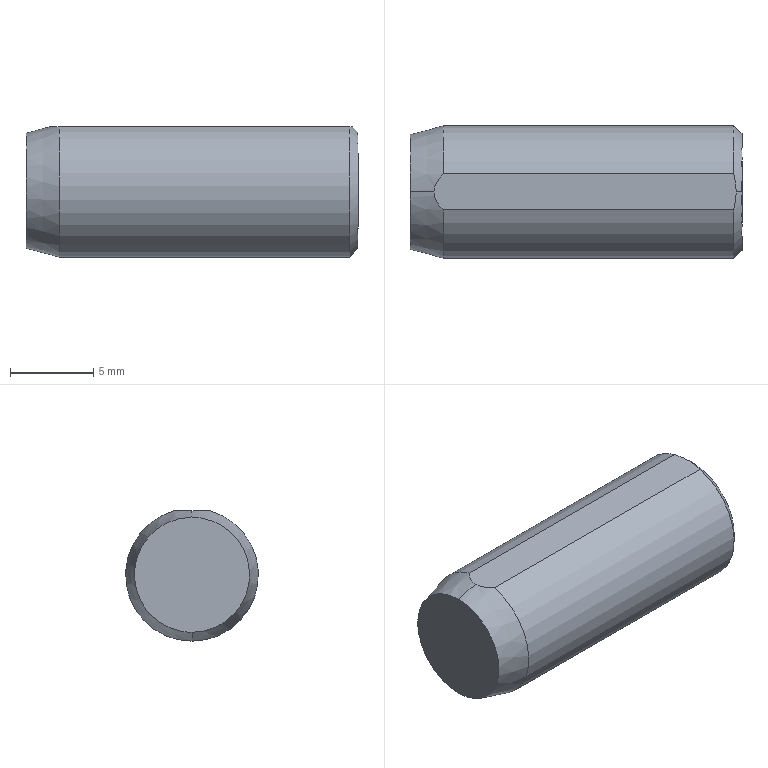Part | STEP file | MSTMS8-20 | 1 solid | 12 faces | box 20 x 8 x 7.85 mm | volume 827.27 mm3 | cone 6 | plane 3 | cylinder 3 | commonest cylinder face diameters 4.2 x2 8 x1
STEP:
#1=CARTESIAN_POINT('',(0.,0.,0.));
#2=DIRECTION('',(0.,0.,1.));
#3=DIRECTION('',(1.,0.,0.));
#4=AXIS2_PLACEMENT_3D('',#1,#2,#3);
#5=CARTESIAN_POINT('',(0.00003804,0.,-3.464));
#6=VERTEX_POINT('',#5);
#7=CARTESIAN_POINT('',(0.00003804,0.,3.464));
#8=VERTEX_POINT('',#7);
#9=CARTESIAN_POINT('',(0.00003804,0.,-3.464));
#10=CARTESIAN_POINT('',(0.,-0.9015,-3.475));
#11=CARTESIAN_POINT('',(0.,-1.808,-3.088));
#12=CARTESIAN_POINT('',(0.,-2.771,-2.129));
#13=CARTESIAN_POINT('',(0.,-3.026,-1.747));
#14=CARTESIAN_POINT('',(0.,-3.372,-0.9087));
#15=CARTESIAN_POINT('',(0.,-3.556,0.));
#16=CARTESIAN_POINT('',(0.,-3.372,0.9087));
#17=CARTESIAN_POINT('',(0.,-3.026,1.747));
#18=CARTESIAN_POINT('',(0.,-2.771,2.129));
#19=CARTESIAN_POINT('',(0.,-1.808,3.088));
#20=CARTESIAN_POINT('',(0.,-0.9015,3.475));
#21=CARTESIAN_POINT('',(0.00003804,0.,3.464));
#22=B_SPLINE_CURVE_WITH_KNOTS('',3,(#9,#10,#11,#12,#13,#14,#15,#16,#17,#18,#19,#20,#21),.UNSPECIFIED.,.F.,.F.,(4,2,2,1,2,2,4),(0.,0.25,0.375,0.5,0.625,0.75,1.),.UNSPECIFIED.);
#23=CARTESIAN_POINT('',(0.,-7.348,7.348));
#24=DIRECTION('',(1.,0.,0.));
#25=DIRECTION('',(0.,0.,-1.));
#26=AXIS2_PLACEMENT_3D('',#23,#24,#25);
#27=PLANE('',#26);
#28=CARTESIAN_POINT('',(10.812,7.348));
#29=CARTESIAN_POINT('',(10.823,6.447));
#30=CARTESIAN_POINT('',(10.436,5.54));
#31=CARTESIAN_POINT('',(9.477,4.577));
#32=CARTESIAN_POINT('',(9.095,4.322));
#33=CARTESIAN_POINT('',(8.257,3.976));
#34=CARTESIAN_POINT('',(7.348,3.792));
#35=CARTESIAN_POINT('',(6.439,3.976));
#36=CARTESIAN_POINT('',(5.601,4.322));
#37=CARTESIAN_POINT('',(5.219,4.577));
#38=CARTESIAN_POINT('',(4.26,5.54));
#39=CARTESIAN_POINT('',(3.873,6.447));
#40=CARTESIAN_POINT('',(3.884,7.348));
#41=B_SPLINE_CURVE_WITH_KNOTS('',3,(#28,#29,#30,#31,#32,#33,#34,#35,#36,#37,#38,#39,#40),.UNSPECIFIED.,.F.,.F.,(4,2,2,1,2,2,4),(0.,0.25,0.375,0.5,0.625,0.75,1.),.UNSPECIFIED.);
#42=(GEOMETRIC_REPRESENTATION_CONTEXT(2)PARAMETRIC_REPRESENTATION_CONTEXT()REPRESENTATION_CONTEXT('',''));
#43=DEFINITIONAL_REPRESENTATION('',(#41),#42);
#44=PCURVE('',#27,#43);
#45=CARTESIAN_POINT('',(-5.702,0.,0.));
#46=DIRECTION('',(1.,0.,0.));
#47=DIRECTION('',(0.,0.,-1.));
#48=AXIS2_PLACEMENT_3D('',#45,#46,#47);
#49=CONICAL_SURFACE('',#48,1.936,0.2618);
#50=CARTESIAN_POINT('',(6.283,5.702));
#51=CARTESIAN_POINT('',(6.26,5.702));
#52=CARTESIAN_POINT('',(6.212,5.702));
#53=CARTESIAN_POINT('',(6.141,5.702));
#54=CARTESIAN_POINT('',(6.07,5.702));
#55=CARTESIAN_POINT('',(5.999,5.702));
#56=CARTESIAN_POINT('',(5.927,5.702));
#57=CARTESIAN_POINT('',(5.856,5.701));
#58=CARTESIAN_POINT('',(5.784,5.701));
#59=CARTESIAN_POINT('',(5.712,5.701));
#60=CARTESIAN_POINT('',(5.64,5.701));
#61=CARTESIAN_POINT('',(5.569,5.702));
#62=CARTESIAN_POINT('',(5.498,5.702));
#63=CARTESIAN_POINT('',(5.426,5.702));
#64=CARTESIAN_POINT('',(5.355,5.702));
#65=CARTESIAN_POINT('',(5.284,5.702));
#66=CARTESIAN_POINT('',(5.213,5.702));
#67=CARTESIAN_POINT('',(5.142,5.702));
#68=CARTESIAN_POINT('',(5.07,5.702));
#69=CARTESIAN_POINT('',(4.999,5.702));
#70=CARTESIAN_POINT('',(4.927,5.702));
#71=CARTESIAN_POINT('',(4.856,5.702));
#72=CARTESIAN_POINT('',(4.784,5.702));
#73=CARTESIAN_POINT('',(4.712,5.702));
#74=CARTESIAN_POINT('',(4.641,5.702));
#75=CARTESIAN_POINT('',(4.569,5.702));
#76=CARTESIAN_POINT('',(4.498,5.702));
#77=CARTESIAN_POINT('',(4.426,5.702));
#78=CARTESIAN_POINT('',(4.355,5.702));
#79=CARTESIAN_POINT('',(4.283,5.702));
#80=CARTESIAN_POINT('',(4.212,5.702));
#81=CARTESIAN_POINT('',(4.141,5.702));
#82=CARTESIAN_POINT('',(4.07,5.702));
#83=CARTESIAN_POINT('',(3.998,5.702));
#84=CARTESIAN_POINT('',(3.927,5.702));
#85=CARTESIAN_POINT('',(3.856,5.702));
#86=CARTESIAN_POINT('',(3.784,5.701));
#87=CARTESIAN_POINT('',(3.713,5.701));
#88=CARTESIAN_POINT('',(3.641,5.701));
#89=CARTESIAN_POINT('',(3.569,5.701));
#90=CARTESIAN_POINT('',(3.498,5.702));
#91=CARTESIAN_POINT('',(3.426,5.702));
#92=CARTESIAN_POINT('',(3.355,5.702));
#93=CARTESIAN_POINT('',(3.284,5.702));
#94=CARTESIAN_POINT('',(3.213,5.702));
#95=CARTESIAN_POINT('',(3.165,5.702));
#96=CARTESIAN_POINT('',(3.142,5.702));
#97=B_SPLINE_CURVE_WITH_KNOTS('',3,(#50,#51,#52,#53,#54,#55,#56,#57,#58,#59,#60,#61,#62,#63,#64,#65,#66,#67,#68,#69,#70,#71,#72,#73,#74,#75,#76,#77,#78,#79,#80,#81,#82,#83,#84,#85,#86,#87,#88,#89,#90,#91,#92,#93,#94,#95,#96),.UNSPECIFIED.,.F.,.F.,(4,1,1,1,1,1,1,1,1,1,1,1,1,1,1,1,1,1,1,1,1,1,1,1,1,1,1,1,1,1,1,1,1,1,1,1,1,1,1,1,1,1,1,1,4),(0.,0.02273,0.04545,0.06818,0.09091,0.1136,0.1364,0.1591,0.1818,0.2045,0.2273,0.25,0.2727,0.2955,0.3182,0.3409,0.3636,0.3864,0.4091,0.4318,0.4545,0.4773,0.5,0.5227,0.5455,0.5682,0.5909,0.6136,0.6364,0.6591,0.6818,0.7045,0.7273,0.75,0.7727,0.7955,0.8182,0.8409,0.8636,0.8864,0.9091,0.9318,0.9545,0.9773,1.),.QUASI_UNIFORM_KNOTS.);
#98=(GEOMETRIC_REPRESENTATION_CONTEXT(2)PARAMETRIC_REPRESENTATION_CONTEXT()REPRESENTATION_CONTEXT('',''));
#99=DEFINITIONAL_REPRESENTATION('',(#97),#98);
#100=PCURVE('',#49,#99);
#101=SURFACE_CURVE('',#22,(#44,#100),.PCURVE_S1.);
#102=EDGE_CURVE('',#6,#8,#101,.T.);
#103=ORIENTED_EDGE('',*,*,#102,.F.);
#104=CARTESIAN_POINT('',(0.00003804,0.,3.464));
#105=CARTESIAN_POINT('',(0.,0.9015,3.475));
#106=CARTESIAN_POINT('',(0.,1.808,3.088));
#107=CARTESIAN_POINT('',(0.,2.771,2.129));
#108=CARTESIAN_POINT('',(0.,3.026,1.747));
#109=CARTESIAN_POINT('',(0.,3.372,0.9087));
#110=CARTESIAN_POINT('',(0.,3.556,0.));
#111=CARTESIAN_POINT('',(0.,3.372,-0.9087));
#112=CARTESIAN_POINT('',(0.,3.026,-1.747));
#113=CARTESIAN_POINT('',(0.,2.771,-2.129));
#114=CARTESIAN_POINT('',(0.,1.808,-3.088));
#115=CARTESIAN_POINT('',(0.,0.9015,-3.475));
#116=CARTESIAN_POINT('',(0.00003804,0.,-3.464));
#117=B_SPLINE_CURVE_WITH_KNOTS('',3,(#104,#105,#106,#107,#108,#109,#110,#111,#112,#113,#114,#115,#116),.UNSPECIFIED.,.F.,.F.,(4,2,2,1,2,2,4),(0.,0.25,0.375,0.5,0.625,0.75,1.),.UNSPECIFIED.);
#118=CARTESIAN_POINT('',(3.884,7.348));
#119=CARTESIAN_POINT('',(3.873,8.25));
#120=CARTESIAN_POINT('',(4.26,9.156));
#121=CARTESIAN_POINT('',(5.219,10.119));
#122=CARTESIAN_POINT('',(5.601,10.374));
#123=CARTESIAN_POINT('',(6.439,10.72));
#124=CARTESIAN_POINT('',(7.348,10.904));
#125=CARTESIAN_POINT('',(8.257,10.72));
#126=CARTESIAN_POINT('',(9.095,10.374));
#127=CARTESIAN_POINT('',(9.477,10.119));
#128=CARTESIAN_POINT('',(10.436,9.156));
#129=CARTESIAN_POINT('',(10.823,8.25));
#130=CARTESIAN_POINT('',(10.812,7.348));
#131=B_SPLINE_CURVE_WITH_KNOTS('',3,(#118,#119,#120,#121,#122,#123,#124,#125,#126,#127,#128,#129,#130),.UNSPECIFIED.,.F.,.F.,(4,2,2,1,2,2,4),(0.,0.25,0.375,0.5,0.625,0.75,1.),.UNSPECIFIED.);
#132=(GEOMETRIC_REPRESENTATION_CONTEXT(2)PARAMETRIC_REPRESENTATION_CONTEXT()REPRESENTATION_CONTEXT('',''));
#133=DEFINITIONAL_REPRESENTATION('',(#131),#132);
#134=PCURVE('',#27,#133);
#135=CARTESIAN_POINT('',(-5.702,0.,0.));
#136=DIRECTION('',(1.,0.,0.));
#137=DIRECTION('',(0.,0.,-1.));
#138=AXIS2_PLACEMENT_3D('',#135,#136,#137);
#139=CONICAL_SURFACE('',#138,1.936,0.2618);
#140=CARTESIAN_POINT('',(3.142,5.702));
#141=CARTESIAN_POINT('',(3.118,5.702));
#142=CARTESIAN_POINT('',(3.071,5.702));
#143=CARTESIAN_POINT('',(3.,5.702));
#144=CARTESIAN_POINT('',(2.928,5.702));
#145=CARTESIAN_POINT('',(2.857,5.702));
#146=CARTESIAN_POINT('',(2.786,5.702));
#147=CARTESIAN_POINT('',(2.714,5.701));
#148=CARTESIAN_POINT('',(2.642,5.701));
#149=CARTESIAN_POINT('',(2.571,5.701));
#150=CARTESIAN_POINT('',(2.499,5.701));
#151=CARTESIAN_POINT('',(2.427,5.702));
#152=CARTESIAN_POINT('',(2.356,5.702));
#153=CARTESIAN_POINT('',(2.285,5.702));
#154=CARTESIAN_POINT('',(2.214,5.702));
#155=CARTESIAN_POINT('',(2.142,5.702));
#156=CARTESIAN_POINT('',(2.071,5.702));
#157=CARTESIAN_POINT('',(2.,5.702));
#158=CARTESIAN_POINT('',(1.929,5.702));
#159=CARTESIAN_POINT('',(1.857,5.702));
#160=CARTESIAN_POINT('',(1.785,5.702));
#161=CARTESIAN_POINT('',(1.714,5.702));
#162=CARTESIAN_POINT('',(1.642,5.702));
#163=CARTESIAN_POINT('',(1.571,5.702));
#164=CARTESIAN_POINT('',(1.499,5.702));
#165=CARTESIAN_POINT('',(1.428,5.702));
#166=CARTESIAN_POINT('',(1.356,5.702));
#167=CARTESIAN_POINT('',(1.285,5.702));
#168=CARTESIAN_POINT('',(1.213,5.702));
#169=CARTESIAN_POINT('',(1.142,5.702));
#170=CARTESIAN_POINT('',(1.07,5.702));
#171=CARTESIAN_POINT('',(0.9992,5.702));
#172=CARTESIAN_POINT('',(0.9281,5.702));
#173=CARTESIAN_POINT('',(0.8569,5.702));
#174=CARTESIAN_POINT('',(0.7857,5.702));
#175=CARTESIAN_POINT('',(0.7143,5.702));
#176=CARTESIAN_POINT('',(0.6427,5.701));
#177=CARTESIAN_POINT('',(0.5711,5.701));
#178=CARTESIAN_POINT('',(0.4994,5.701));
#179=CARTESIAN_POINT('',(0.4276,5.701));
#180=CARTESIAN_POINT('',(0.356,5.702));
#181=CARTESIAN_POINT('',(0.2845,5.702));
#182=CARTESIAN_POINT('',(0.2132,5.702));
#183=CARTESIAN_POINT('',(0.142,5.702));
#184=CARTESIAN_POINT('',(0.07096,5.702));
#185=CARTESIAN_POINT('',(0.02365,5.702));
#186=CARTESIAN_POINT('',(0.,5.702));
#187=B_SPLINE_CURVE_WITH_KNOTS('',3,(#140,#141,#142,#143,#144,#145,#146,#147,#148,#149,#150,#151,#152,#153,#154,#155,#156,#157,#158,#159,#160,#161,#162,#163,#164,#165,#166,#167,#168,#169,#170,#171,#172,#173,#174,#175,#176,#177,#178,#179,#180,#181,#182,#183,#184,#185,#186),.UNSPECIFIED.,.F.,.F.,(4,1,1,1,1,1,1,1,1,1,1,1,1,1,1,1,1,1,1,1,1,1,1,1,1,1,1,1,1,1,1,1,1,1,1,1,1,1,1,1,1,1,1,1,4),(0.,0.02273,0.04545,0.06818,0.09091,0.1136,0.1364,0.1591,0.1818,0.2045,0.2273,0.25,0.2727,0.2955,0.3182,0.3409,0.3636,0.3864,0.4091,0.4318,0.4545,0.4773,0.5,0.5227,0.5455,0.5682,0.5909,0.6136,0.6364,0.6591,0.6818,0.7045,0.7273,0.75,0.7727,0.7955,0.8182,0.8409,0.8636,0.8864,0.9091,0.9318,0.9545,0.9773,1.),.QUASI_UNIFORM_KNOTS.);
#188=(GEOMETRIC_REPRESENTATION_CONTEXT(2)PARAMETRIC_REPRESENTATION_CONTEXT()REPRESENTATION_CONTEXT('',''));
#189=DEFINITIONAL_REPRESENTATION('',(#187),#188);
#190=PCURVE('',#139,#189);
#191=SURFACE_CURVE('',#117,(#134,#190),.PCURVE_S1.);
#192=EDGE_CURVE('',#8,#6,#191,.T.);
#193=ORIENTED_EDGE('',*,*,#192,.F.);
#194=EDGE_LOOP('',(#103,#193));
#195=FACE_BOUND('',#194,.F.);
#196=ADVANCED_FACE('',(#195),#27,.F.);
#197=CARTESIAN_POINT('',(1.441,0.00000021,3.85));
#198=VERTEX_POINT('',#197);
#199=CARTESIAN_POINT('',(0.00003804,0.,3.464));
#200=DIRECTION('',(0.9659,0.000000141,0.2588));
#201=VECTOR('',#200,1.);
#202=LINE('',#199,#201);
#203=CARTESIAN_POINT('',(3.142,5.702));
#204=DIRECTION('',(-0.000000038,1.));
#205=VECTOR('',#204,1.);
#206=LINE('',#203,#205);
#207=(GEOMETRIC_REPRESENTATION_CONTEXT(2)PARAMETRIC_REPRESENTATION_CONTEXT()REPRESENTATION_CONTEXT('',''));
#208=DEFINITIONAL_REPRESENTATION('',(#206),#207);
#209=PCURVE('',#49,#208);
#210=CARTESIAN_POINT('',(3.142,5.702));
#211=DIRECTION('',(-0.000000038,1.));
#212=VECTOR('',#211,1.);
#213=LINE('',#210,#212);
#214=(GEOMETRIC_REPRESENTATION_CONTEXT(2)PARAMETRIC_REPRESENTATION_CONTEXT()REPRESENTATION_CONTEXT('',''));
#215=DEFINITIONAL_REPRESENTATION('',(#213),#214);
#216=PCURVE('',#139,#215);
#217=SURFACE_CURVE('',#202,(#209,#216),.PCURVE_S1.);
#218=EDGE_CURVE('',#8,#198,#217,.T.);
#219=ORIENTED_EDGE('',*,*,#218,.F.);
#220=ORIENTED_EDGE('',*,*,#102,.F.);
#221=CARTESIAN_POINT('',(2.,-0.000000145,-4.));
#222=VERTEX_POINT('',#221);
#223=CARTESIAN_POINT('',(0.00003804,0.,-3.464));
#224=CARTESIAN_POINT('',(0.667,0.,-3.643));
#225=CARTESIAN_POINT('',(1.334,0.,-3.821));
#226=CARTESIAN_POINT('',(2.,-0.000000145,-4.));
#227=B_SPLINE_CURVE_WITH_KNOTS('',3,(#223,#224,#225,#226),.UNSPECIFIED.,.F.,.F.,(4,4),(0.,1.),.PIECEWISE_BEZIER_KNOTS.);
#228=CARTESIAN_POINT('',(6.283,5.702));
#229=CARTESIAN_POINT('',(6.283,5.732));
#230=CARTESIAN_POINT('',(6.283,5.793));
#231=CARTESIAN_POINT('',(6.283,5.884));
#232=CARTESIAN_POINT('',(6.283,5.975));
#233=CARTESIAN_POINT('',(6.283,6.066));
#234=CARTESIAN_POINT('',(6.283,6.157));
#235=CARTESIAN_POINT('',(6.283,6.247));
#236=CARTESIAN_POINT('',(6.283,6.338));
#237=CARTESIAN_POINT('',(6.283,6.429));
#238=CARTESIAN_POINT('',(6.283,6.52));
#239=CARTESIAN_POINT('',(6.283,6.611));
#240=CARTESIAN_POINT('',(6.283,6.702));
#241=CARTESIAN_POINT('',(6.283,6.793));
#242=CARTESIAN_POINT('',(6.283,6.884));
#243=CARTESIAN_POINT('',(6.283,6.975));
#244=CARTESIAN_POINT('',(6.283,7.066));
#245=CARTESIAN_POINT('',(6.283,7.157));
#246=CARTESIAN_POINT('',(6.283,7.248));
#247=CARTESIAN_POINT('',(6.283,7.338));
#248=CARTESIAN_POINT('',(6.283,7.429));
#249=CARTESIAN_POINT('',(6.283,7.52));
#250=CARTESIAN_POINT('',(6.283,7.611));
#251=CARTESIAN_POINT('',(6.283,7.672));
#252=CARTESIAN_POINT('',(6.283,7.702));
#253=B_SPLINE_CURVE_WITH_KNOTS('',3,(#228,#229,#230,#231,#232,#233,#234,#235,#236,#237,#238,#239,#240,#241,#242,#243,#244,#245,#246,#247,#248,#249,#250,#251,#252),.UNSPECIFIED.,.F.,.F.,(4,1,1,1,1,1,1,1,1,1,1,1,1,1,1,1,1,1,1,1,1,1,4),(0.,0.04545,0.09091,0.1364,0.1818,0.2273,0.2727,0.3182,0.3636,0.4091,0.4545,0.5,0.5455,0.5909,0.6364,0.6818,0.7273,0.7727,0.8182,0.8636,0.9091,0.9545,1.),.QUASI_UNIFORM_KNOTS.);
#254=(GEOMETRIC_REPRESENTATION_CONTEXT(2)PARAMETRIC_REPRESENTATION_CONTEXT()REPRESENTATION_CONTEXT('',''));
#255=DEFINITIONAL_REPRESENTATION('',(#253),#254);
#256=PCURVE('',#49,#255);
#257=CARTESIAN_POINT('',(0.,5.702));
#258=CARTESIAN_POINT('',(0.,5.732));
#259=CARTESIAN_POINT('',(0.,5.793));
#260=CARTESIAN_POINT('',(0.,5.884));
#261=CARTESIAN_POINT('',(0.,5.975));
#262=CARTESIAN_POINT('',(0.,6.066));
#263=CARTESIAN_POINT('',(0.,6.157));
#264=CARTESIAN_POINT('',(-0.000000001,6.247));
#265=CARTESIAN_POINT('',(-0.000000001,6.338));
#266=CARTESIAN_POINT('',(-0.000000002,6.429));
#267=CARTESIAN_POINT('',(-0.000000003,6.52));
#268=CARTESIAN_POINT('',(-0.000000004,6.611));
#269=CARTESIAN_POINT('',(-0.000000005,6.702));
#270=CARTESIAN_POINT('',(-0.000000006,6.793));
#271=CARTESIAN_POINT('',(-0.000000008,6.884));
#272=CARTESIAN_POINT('',(-0.00000001,6.975));
#273=CARTESIAN_POINT('',(-0.000000012,7.066));
#274=CARTESIAN_POINT('',(-0.000000014,7.157));
#275=CARTESIAN_POINT('',(-0.000000017,7.248));
#276=CARTESIAN_POINT('',(-0.00000002,7.338));
#277=CARTESIAN_POINT('',(-0.000000024,7.429));
#278=CARTESIAN_POINT('',(-0.000000028,7.52));
#279=CARTESIAN_POINT('',(-0.000000032,7.611));
#280=CARTESIAN_POINT('',(-0.000000035,7.672));
#281=CARTESIAN_POINT('',(-0.000000036,7.702));
#282=B_SPLINE_CURVE_WITH_KNOTS('',3,(#257,#258,#259,#260,#261,#262,#263,#264,#265,#266,#267,#268,#269,#270,#271,#272,#273,#274,#275,#276,#277,#278,#279,#280,#281),.UNSPECIFIED.,.F.,.F.,(4,1,1,1,1,1,1,1,1,1,1,1,1,1,1,1,1,1,1,1,1,1,4),(0.,0.04545,0.09091,0.1364,0.1818,0.2273,0.2727,0.3182,0.3636,0.4091,0.4545,0.5,0.5455,0.5909,0.6364,0.6818,0.7273,0.7727,0.8182,0.8636,0.9091,0.9545,1.),.QUASI_UNIFORM_KNOTS.);
#283=(GEOMETRIC_REPRESENTATION_CONTEXT(2)PARAMETRIC_REPRESENTATION_CONTEXT()REPRESENTATION_CONTEXT('',''));
#284=DEFINITIONAL_REPRESENTATION('',(#282),#283);
#285=PCURVE('',#139,#284);
#286=SURFACE_CURVE('',#227,(#256,#285),.PCURVE_S1.);
#287=EDGE_CURVE('',#6,#222,#286,.T.);
#288=ORIENTED_EDGE('',*,*,#287,.T.);
#289=CARTESIAN_POINT('',(2.001,-1.085,3.85));
#290=VERTEX_POINT('',#289);
#291=CARTESIAN_POINT('',(2.001,0.,0.));
#292=DIRECTION('',(-1.,0.,0.));
#293=DIRECTION('',(0.,-0.000000036,-1.));
#294=AXIS2_PLACEMENT_3D('',#291,#292,#293);
#295=CIRCLE('',#294,4.);
#296=CARTESIAN_POINT('',(6.283,7.703));
#297=DIRECTION('',(-1.,0.));
#298=VECTOR('',#297,1.);
#299=LINE('',#296,#298);
#300=(GEOMETRIC_REPRESENTATION_CONTEXT(2)PARAMETRIC_REPRESENTATION_CONTEXT()REPRESENTATION_CONTEXT('',''));
#301=DEFINITIONAL_REPRESENTATION('',(#299),#300);
#302=PCURVE('',#49,#301);
#303=CARTESIAN_POINT('',(10.75,0.,0.));
#304=DIRECTION('',(1.,0.,0.));
#305=DIRECTION('',(0.,0.008727,1.));
#306=AXIS2_PLACEMENT_3D('',#303,#304,#305);
#307=CYLINDRICAL_SURFACE('',#306,4.);
#308=CARTESIAN_POINT('',(3.15,-8.749));
#309=DIRECTION('',(-1.,0.));
#310=VECTOR('',#309,1.);
#311=LINE('',#308,#310);
#312=(GEOMETRIC_REPRESENTATION_CONTEXT(2)PARAMETRIC_REPRESENTATION_CONTEXT()REPRESENTATION_CONTEXT('',''));
#313=DEFINITIONAL_REPRESENTATION('',(#311),#312);
#314=PCURVE('',#307,#313);
#315=SURFACE_CURVE('',#295,(#302,#314),.PCURVE_S1.);
#316=EDGE_CURVE('',#222,#290,#315,.T.);
#317=ORIENTED_EDGE('',*,*,#316,.T.);
#318=CARTESIAN_POINT('',(1.441,0.00000021,3.85));
#319=CARTESIAN_POINT('',(1.441,-0.4288,3.85));
#320=CARTESIAN_POINT('',(1.711,-0.7982,3.85));
#321=CARTESIAN_POINT('',(2.001,-1.085,3.85));
#322=B_SPLINE_CURVE_WITH_KNOTS('',3,(#318,#319,#320,#321),.UNSPECIFIED.,.F.,.F.,(4,4),(0.,1.),.PIECEWISE_BEZIER_KNOTS.);
#323=CARTESIAN_POINT('',(3.142,7.143));
#324=CARTESIAN_POINT('',(3.147,7.143));
#325=CARTESIAN_POINT('',(3.157,7.144));
#326=CARTESIAN_POINT('',(3.172,7.149));
#327=CARTESIAN_POINT('',(3.186,7.157));
#328=CARTESIAN_POINT('',(3.201,7.167));
#329=CARTESIAN_POINT('',(3.215,7.181));
#330=CARTESIAN_POINT('',(3.229,7.197));
#331=CARTESIAN_POINT('',(3.243,7.216));
#332=CARTESIAN_POINT('',(3.256,7.237));
#333=CARTESIAN_POINT('',(3.269,7.261));
#334=CARTESIAN_POINT('',(3.282,7.286));
#335=CARTESIAN_POINT('',(3.295,7.314));
#336=CARTESIAN_POINT('',(3.308,7.343));
#337=CARTESIAN_POINT('',(3.32,7.374));
#338=CARTESIAN_POINT('',(3.332,7.406));
#339=CARTESIAN_POINT('',(3.343,7.44));
#340=CARTESIAN_POINT('',(3.355,7.475));
#341=CARTESIAN_POINT('',(3.366,7.511));
#342=CARTESIAN_POINT('',(3.376,7.548));
#343=CARTESIAN_POINT('',(3.387,7.586));
#344=CARTESIAN_POINT('',(3.397,7.624));
#345=CARTESIAN_POINT('',(3.407,7.663));
#346=CARTESIAN_POINT('',(3.413,7.689));
#347=CARTESIAN_POINT('',(3.416,7.703));
#348=B_SPLINE_CURVE_WITH_KNOTS('',3,(#323,#324,#325,#326,#327,#328,#329,#330,#331,#332,#333,#334,#335,#336,#337,#338,#339,#340,#341,#342,#343,#344,#345,#346,#347),.UNSPECIFIED.,.F.,.F.,(4,1,1,1,1,1,1,1,1,1,1,1,1,1,1,1,1,1,1,1,1,1,4),(0.,0.04545,0.09091,0.1364,0.1818,0.2273,0.2727,0.3182,0.3636,0.4091,0.4545,0.5,0.5455,0.5909,0.6364,0.6818,0.7273,0.7727,0.8182,0.8636,0.9091,0.9545,1.),.QUASI_UNIFORM_KNOTS.);
#349=(GEOMETRIC_REPRESENTATION_CONTEXT(2)PARAMETRIC_REPRESENTATION_CONTEXT()REPRESENTATION_CONTEXT('',''));
#350=DEFINITIONAL_REPRESENTATION('',(#348),#349);
#351=PCURVE('',#49,#350);
#352=CARTESIAN_POINT('',(-3.208,-13.753,3.85));
#353=DIRECTION('',(0.,0.,-1.));
#354=DIRECTION('',(0.,1.,0.));
#355=AXIS2_PLACEMENT_3D('',#352,#353,#354);
#356=PLANE('',#355);
#357=CARTESIAN_POINT('',(13.753,4.649));
#358=CARTESIAN_POINT('',(13.324,4.648));
#359=CARTESIAN_POINT('',(12.955,4.919));
#360=CARTESIAN_POINT('',(12.668,5.209));
#361=B_SPLINE_CURVE_WITH_KNOTS('',3,(#357,#358,#359,#360),.UNSPECIFIED.,.F.,.F.,(4,4),(0.,1.),.PIECEWISE_BEZIER_KNOTS.);
#362=(GEOMETRIC_REPRESENTATION_CONTEXT(2)PARAMETRIC_REPRESENTATION_CONTEXT()REPRESENTATION_CONTEXT('',''));
#363=DEFINITIONAL_REPRESENTATION('',(#361),#362);
#364=PCURVE('',#356,#363);
#365=SURFACE_CURVE('',#322,(#351,#364),.PCURVE_S1.);
#366=EDGE_CURVE('',#198,#290,#365,.T.);
#367=ORIENTED_EDGE('',*,*,#366,.F.);
#368=EDGE_LOOP('',(#219,#220,#288,#317,#367));
#369=FACE_BOUND('',#368,.T.);
#370=ADVANCED_FACE('',(#369),#49,.T.);
#371=CARTESIAN_POINT('',(19.65,0.000000117,3.85));
#372=VERTEX_POINT('',#371);
#373=CARTESIAN_POINT('',(19.5,1.085,3.85));
#374=VERTEX_POINT('',#373);
#375=CARTESIAN_POINT('',(19.65,0.000000117,3.85));
#376=CARTESIAN_POINT('',(19.65,0.3664,3.85));
#377=CARTESIAN_POINT('',(19.596,0.7319,3.85));
#378=CARTESIAN_POINT('',(19.5,1.085,3.85));
#379=B_SPLINE_CURVE_WITH_KNOTS('',3,(#375,#376,#377,#378),.UNSPECIFIED.,.F.,.F.,(4,4),(0.,1.),.PIECEWISE_BEZIER_KNOTS.);
#380=CARTESIAN_POINT('',(13.753,22.858));
#381=CARTESIAN_POINT('',(14.12,22.858));
#382=CARTESIAN_POINT('',(14.485,22.804));
#383=CARTESIAN_POINT('',(14.838,22.708));
#384=B_SPLINE_CURVE_WITH_KNOTS('',3,(#380,#381,#382,#383),.UNSPECIFIED.,.F.,.F.,(4,4),(0.,1.),.PIECEWISE_BEZIER_KNOTS.);
#385=(GEOMETRIC_REPRESENTATION_CONTEXT(2)PARAMETRIC_REPRESENTATION_CONTEXT()REPRESENTATION_CONTEXT('',''));
#386=DEFINITIONAL_REPRESENTATION('',(#384),#385);
#387=PCURVE('',#356,#386);
#388=CARTESIAN_POINT('',(-976.5,0.,0.));
#389=DIRECTION('',(-1.,0.,0.));
#390=DIRECTION('',(0.,0.,-1.));
#391=AXIS2_PLACEMENT_3D('',#388,#389,#390);
#392=CONICAL_SURFACE('',#391,999.941,0.7854);
#393=CARTESIAN_POINT('',(3.142,-996.15));
#394=CARTESIAN_POINT('',(3.146,-996.15));
#395=CARTESIAN_POINT('',(3.155,-996.15));
#396=CARTESIAN_POINT('',(3.168,-996.149));
#397=CARTESIAN_POINT('',(3.18,-996.147));
#398=CARTESIAN_POINT('',(3.193,-996.145));
#399=CARTESIAN_POINT('',(3.206,-996.142));
#400=CARTESIAN_POINT('',(3.219,-996.138));
#401=CARTESIAN_POINT('',(3.232,-996.134));
#402=CARTESIAN_POINT('',(3.245,-996.129));
#403=CARTESIAN_POINT('',(3.258,-996.124));
#404=CARTESIAN_POINT('',(3.27,-996.118));
#405=CARTESIAN_POINT('',(3.283,-996.111));
#406=CARTESIAN_POINT('',(3.295,-996.104));
#407=CARTESIAN_POINT('',(3.308,-996.096));
#408=CARTESIAN_POINT('',(3.32,-996.088));
#409=CARTESIAN_POINT('',(3.333,-996.079));
#410=CARTESIAN_POINT('',(3.345,-996.069));
#411=CARTESIAN_POINT('',(3.357,-996.059));
#412=CARTESIAN_POINT('',(3.369,-996.048));
#413=CARTESIAN_POINT('',(3.381,-996.037));
#414=CARTESIAN_POINT('',(3.393,-996.025));
#415=CARTESIAN_POINT('',(3.405,-996.013));
#416=CARTESIAN_POINT('',(3.412,-996.004));
#417=CARTESIAN_POINT('',(3.416,-996.));
#418=B_SPLINE_CURVE_WITH_KNOTS('',3,(#393,#394,#395,#396,#397,#398,#399,#400,#401,#402,#403,#404,#405,#406,#407,#408,#409,#410,#411,#412,#413,#414,#415,#416,#417),.UNSPECIFIED.,.F.,.F.,(4,1,1,1,1,1,1,1,1,1,1,1,1,1,1,1,1,1,1,1,1,1,4),(0.,0.04545,0.09091,0.1364,0.1818,0.2273,0.2727,0.3182,0.3636,0.4091,0.4545,0.5,0.5455,0.5909,0.6364,0.6818,0.7273,0.7727,0.8182,0.8636,0.9091,0.9545,1.),.QUASI_UNIFORM_KNOTS.);
#419=(GEOMETRIC_REPRESENTATION_CONTEXT(2)PARAMETRIC_REPRESENTATION_CONTEXT()REPRESENTATION_CONTEXT('',''));
#420=DEFINITIONAL_REPRESENTATION('',(#418),#419);
#421=PCURVE('',#392,#420);
#422=SURFACE_CURVE('',#379,(#387,#421),.PCURVE_S1.);
#423=EDGE_CURVE('',#372,#374,#422,.T.);
#424=ORIENTED_EDGE('',*,*,#423,.F.);
#425=CARTESIAN_POINT('',(19.5,-1.085,3.85));
#426=VERTEX_POINT('',#425);
#427=CARTESIAN_POINT('',(19.5,-1.085,3.85));
#428=CARTESIAN_POINT('',(19.596,-0.7319,3.85));
#429=CARTESIAN_POINT('',(19.65,-0.3664,3.85));
#430=CARTESIAN_POINT('',(19.65,0.000000117,3.85));
#431=B_SPLINE_CURVE_WITH_KNOTS('',3,(#427,#428,#429,#430),.UNSPECIFIED.,.F.,.F.,(4,4),(0.,1.),.PIECEWISE_BEZIER_KNOTS.);
#432=CARTESIAN_POINT('',(12.668,22.708));
#433=CARTESIAN_POINT('',(13.021,22.804));
#434=CARTESIAN_POINT('',(13.387,22.858));
#435=CARTESIAN_POINT('',(13.753,22.858));
#436=B_SPLINE_CURVE_WITH_KNOTS('',3,(#432,#433,#434,#435),.UNSPECIFIED.,.F.,.F.,(4,4),(0.,1.),.PIECEWISE_BEZIER_KNOTS.);
#437=(GEOMETRIC_REPRESENTATION_CONTEXT(2)PARAMETRIC_REPRESENTATION_CONTEXT()REPRESENTATION_CONTEXT('',''));
#438=DEFINITIONAL_REPRESENTATION('',(#436),#437);
#439=PCURVE('',#356,#438);
#440=CARTESIAN_POINT('',(-976.5,0.,0.));
#441=DIRECTION('',(-1.,0.,0.));
#442=DIRECTION('',(0.,0.,-1.));
#443=AXIS2_PLACEMENT_3D('',#440,#441,#442);
#444=CONICAL_SURFACE('',#443,999.941,0.7854);
#445=CARTESIAN_POINT('',(2.867,-996.));
#446=CARTESIAN_POINT('',(2.871,-996.004));
#447=CARTESIAN_POINT('',(2.878,-996.013));
#448=CARTESIAN_POINT('',(2.89,-996.025));
#449=CARTESIAN_POINT('',(2.902,-996.037));
#450=CARTESIAN_POINT('',(2.914,-996.048));
#451=CARTESIAN_POINT('',(2.926,-996.059));
#452=CARTESIAN_POINT('',(2.938,-996.069));
#453=CARTESIAN_POINT('',(2.951,-996.079));
#454=CARTESIAN_POINT('',(2.963,-996.088));
#455=CARTESIAN_POINT('',(2.975,-996.096));
#456=CARTESIAN_POINT('',(2.988,-996.104));
#457=CARTESIAN_POINT('',(3.,-996.111));
#458=CARTESIAN_POINT('',(3.013,-996.118));
#459=CARTESIAN_POINT('',(3.026,-996.124));
#460=CARTESIAN_POINT('',(3.038,-996.129));
#461=CARTESIAN_POINT('',(3.051,-996.134));
#462=CARTESIAN_POINT('',(3.064,-996.138));
#463=CARTESIAN_POINT('',(3.077,-996.142));
#464=CARTESIAN_POINT('',(3.09,-996.145));
#465=CARTESIAN_POINT('',(3.103,-996.147));
#466=CARTESIAN_POINT('',(3.116,-996.149));
#467=CARTESIAN_POINT('',(3.129,-996.15));
#468=CARTESIAN_POINT('',(3.137,-996.15));
#469=CARTESIAN_POINT('',(3.142,-996.15));
#470=B_SPLINE_CURVE_WITH_KNOTS('',3,(#445,#446,#447,#448,#449,#450,#451,#452,#453,#454,#455,#456,#457,#458,#459,#460,#461,#462,#463,#464,#465,#466,#467,#468,#469),.UNSPECIFIED.,.F.,.F.,(4,1,1,1,1,1,1,1,1,1,1,1,1,1,1,1,1,1,1,1,1,1,4),(0.,0.04545,0.09091,0.1364,0.1818,0.2273,0.2727,0.3182,0.3636,0.4091,0.4545,0.5,0.5455,0.5909,0.6364,0.6818,0.7273,0.7727,0.8182,0.8636,0.9091,0.9545,1.),.QUASI_UNIFORM_KNOTS.);
#471=(GEOMETRIC_REPRESENTATION_CONTEXT(2)PARAMETRIC_REPRESENTATION_CONTEXT()REPRESENTATION_CONTEXT('',''));
#472=DEFINITIONAL_REPRESENTATION('',(#470),#471);
#473=PCURVE('',#444,#472);
#474=SURFACE_CURVE('',#431,(#439,#473),.PCURVE_S1.);
#475=EDGE_CURVE('',#426,#372,#474,.T.);
#476=ORIENTED_EDGE('',*,*,#475,.F.);
#477=CARTESIAN_POINT('',(2.001,-1.085,3.85));
#478=DIRECTION('',(1.,0.,0.));
#479=VECTOR('',#478,1.);
#480=LINE('',#477,#479);
#481=CARTESIAN_POINT('',(12.668,5.209));
#482=DIRECTION('',(0.,1.));
#483=VECTOR('',#482,1.);
#484=LINE('',#481,#483);
#485=(GEOMETRIC_REPRESENTATION_CONTEXT(2)PARAMETRIC_REPRESENTATION_CONTEXT()REPRESENTATION_CONTEXT('',''));
#486=DEFINITIONAL_REPRESENTATION('',(#484),#485);
#487=PCURVE('',#356,#486);
#488=CARTESIAN_POINT('',(0.2835,-8.749));
#489=DIRECTION('',(0.,1.));
#490=VECTOR('',#489,1.);
#491=LINE('',#488,#490);
#492=(GEOMETRIC_REPRESENTATION_CONTEXT(2)PARAMETRIC_REPRESENTATION_CONTEXT()REPRESENTATION_CONTEXT('',''));
#493=DEFINITIONAL_REPRESENTATION('',(#491),#492);
#494=PCURVE('',#307,#493);
#495=SURFACE_CURVE('',#480,(#487,#494),.PCURVE_S1.);
#496=EDGE_CURVE('',#290,#426,#495,.T.);
#497=ORIENTED_EDGE('',*,*,#496,.F.);
#498=ORIENTED_EDGE('',*,*,#366,.F.);
#499=CARTESIAN_POINT('',(2.001,1.085,3.85));
#500=VERTEX_POINT('',#499);
#501=CARTESIAN_POINT('',(2.001,1.085,3.85));
#502=CARTESIAN_POINT('',(1.711,0.7982,3.85));
#503=CARTESIAN_POINT('',(1.441,0.4288,3.85));
#504=CARTESIAN_POINT('',(1.441,0.00000021,3.85));
#505=B_SPLINE_CURVE_WITH_KNOTS('',3,(#501,#502,#503,#504),.UNSPECIFIED.,.F.,.F.,(4,4),(0.,1.),.PIECEWISE_BEZIER_KNOTS.);
#506=CARTESIAN_POINT('',(14.838,5.209));
#507=CARTESIAN_POINT('',(14.551,4.919));
#508=CARTESIAN_POINT('',(14.182,4.648));
#509=CARTESIAN_POINT('',(13.753,4.649));
#510=B_SPLINE_CURVE_WITH_KNOTS('',3,(#506,#507,#508,#509),.UNSPECIFIED.,.F.,.F.,(4,4),(0.,1.),.PIECEWISE_BEZIER_KNOTS.);
#511=(GEOMETRIC_REPRESENTATION_CONTEXT(2)PARAMETRIC_REPRESENTATION_CONTEXT()REPRESENTATION_CONTEXT('',''));
#512=DEFINITIONAL_REPRESENTATION('',(#510),#511);
#513=PCURVE('',#356,#512);
#514=CARTESIAN_POINT('',(2.867,7.703));
#515=CARTESIAN_POINT('',(2.87,7.689));
#516=CARTESIAN_POINT('',(2.876,7.663));
#517=CARTESIAN_POINT('',(2.886,7.624));
#518=CARTESIAN_POINT('',(2.896,7.586));
#519=CARTESIAN_POINT('',(2.907,7.548));
#520=CARTESIAN_POINT('',(2.918,7.511));
#521=CARTESIAN_POINT('',(2.929,7.475));
#522=CARTESIAN_POINT('',(2.94,7.44));
#523=CARTESIAN_POINT('',(2.952,7.406));
#524=CARTESIAN_POINT('',(2.963,7.374));
#525=CARTESIAN_POINT('',(2.976,7.343));
#526=CARTESIAN_POINT('',(2.988,7.314));
#527=CARTESIAN_POINT('',(3.001,7.286));
#528=CARTESIAN_POINT('',(3.014,7.261));
#529=CARTESIAN_POINT('',(3.027,7.237));
#530=CARTESIAN_POINT('',(3.04,7.216));
#531=CARTESIAN_POINT('',(3.054,7.197));
#532=CARTESIAN_POINT('',(3.068,7.181));
#533=CARTESIAN_POINT('',(3.082,7.167));
#534=CARTESIAN_POINT('',(3.097,7.157));
#535=CARTESIAN_POINT('',(3.112,7.149));
#536=CARTESIAN_POINT('',(3.126,7.144));
#537=CARTESIAN_POINT('',(3.137,7.143));
#538=CARTESIAN_POINT('',(3.142,7.143));
#539=B_SPLINE_CURVE_WITH_KNOTS('',3,(#514,#515,#516,#517,#518,#519,#520,#521,#522,#523,#524,#525,#526,#527,#528,#529,#530,#531,#532,#533,#534,#535,#536,#537,#538),.UNSPECIFIED.,.F.,.F.,(4,1,1,1,1,1,1,1,1,1,1,1,1,1,1,1,1,1,1,1,1,1,4),(0.,0.04545,0.09091,0.1364,0.1818,0.2273,0.2727,0.3182,0.3636,0.4091,0.4545,0.5,0.5455,0.5909,0.6364,0.6818,0.7273,0.7727,0.8182,0.8636,0.9091,0.9545,1.),.QUASI_UNIFORM_KNOTS.);
#540=(GEOMETRIC_REPRESENTATION_CONTEXT(2)PARAMETRIC_REPRESENTATION_CONTEXT()REPRESENTATION_CONTEXT('',''));
#541=DEFINITIONAL_REPRESENTATION('',(#539),#540);
#542=PCURVE('',#139,#541);
#543=SURFACE_CURVE('',#505,(#513,#542),.PCURVE_S1.);
#544=EDGE_CURVE('',#500,#198,#543,.T.);
#545=ORIENTED_EDGE('',*,*,#544,.F.);
#546=CARTESIAN_POINT('',(2.001,1.085,3.85));
#547=DIRECTION('',(1.,0.,0.));
#548=VECTOR('',#547,1.);
#549=LINE('',#546,#548);
#550=CARTESIAN_POINT('',(14.838,5.209));
#551=DIRECTION('',(0.,1.));
#552=VECTOR('',#551,1.);
#553=LINE('',#550,#552);
#554=(GEOMETRIC_REPRESENTATION_CONTEXT(2)PARAMETRIC_REPRESENTATION_CONTEXT()REPRESENTATION_CONTEXT('',''));
#555=DEFINITIONAL_REPRESENTATION('',(#553),#554);
#556=PCURVE('',#356,#555);
#557=CARTESIAN_POINT('',(6.017,-8.749));
#558=DIRECTION('',(0.,1.));
#559=VECTOR('',#558,1.);
#560=LINE('',#557,#559);
#561=(GEOMETRIC_REPRESENTATION_CONTEXT(2)PARAMETRIC_REPRESENTATION_CONTEXT()REPRESENTATION_CONTEXT('',''));
#562=DEFINITIONAL_REPRESENTATION('',(#560),#561);
#563=PCURVE('',#307,#562);
#564=SURFACE_CURVE('',#549,(#556,#563),.PCURVE_S1.);
#565=EDGE_CURVE('',#500,#374,#564,.T.);
#566=ORIENTED_EDGE('',*,*,#565,.T.);
#567=EDGE_LOOP('',(#424,#476,#497,#498,#545,#566));
#568=FACE_BOUND('',#567,.F.);
#569=ADVANCED_FACE('',(#568),#356,.F.);
#570=CARTESIAN_POINT('',(20.,0.,3.5));
#571=VERTEX_POINT('',#570);
#572=CARTESIAN_POINT('',(20.,0.,3.5));
#573=DIRECTION('',(-0.7071,0.000000236,0.7071));
#574=VECTOR('',#573,1.);
#575=LINE('',#572,#574);
#576=CARTESIAN_POINT('',(3.142,-996.5));
#577=DIRECTION('',(0.000000087,1.));
#578=VECTOR('',#577,1.);
#579=LINE('',#576,#578);
#580=(GEOMETRIC_REPRESENTATION_CONTEXT(2)PARAMETRIC_REPRESENTATION_CONTEXT()REPRESENTATION_CONTEXT('',''));
#581=DEFINITIONAL_REPRESENTATION('',(#579),#580);
#582=PCURVE('',#392,#581);
#583=CARTESIAN_POINT('',(3.142,-996.5));
#584=DIRECTION('',(0.000000087,1.));
#585=VECTOR('',#584,1.);
#586=LINE('',#583,#585);
#587=(GEOMETRIC_REPRESENTATION_CONTEXT(2)PARAMETRIC_REPRESENTATION_CONTEXT()REPRESENTATION_CONTEXT('',''));
#588=DEFINITIONAL_REPRESENTATION('',(#586),#587);
#589=PCURVE('',#444,#588);
#590=SURFACE_CURVE('',#575,(#582,#589),.PCURVE_S1.);
#591=EDGE_CURVE('',#571,#372,#590,.T.);
#592=ORIENTED_EDGE('',*,*,#591,.F.);
#593=CARTESIAN_POINT('',(20.,0.,-3.5));
#594=VERTEX_POINT('',#593);
#595=CARTESIAN_POINT('',(20.,0.,-3.5));
#596=CARTESIAN_POINT('',(20.,0.9108,-3.511));
#597=CARTESIAN_POINT('',(20.,1.827,-3.12));
#598=CARTESIAN_POINT('',(20.,2.8,-2.151));
#599=CARTESIAN_POINT('',(20.,3.057,-1.765));
#600=CARTESIAN_POINT('',(20.,3.407,-0.9182));
#601=CARTESIAN_POINT('',(20.,3.593,0.));
#602=CARTESIAN_POINT('',(20.,3.407,0.9182));
#603=CARTESIAN_POINT('',(20.,3.057,1.765));
#604=CARTESIAN_POINT('',(20.,2.8,2.151));
#605=CARTESIAN_POINT('',(20.,1.827,3.12));
#606=CARTESIAN_POINT('',(20.,0.9108,3.511));
#607=CARTESIAN_POINT('',(20.,0.,3.5));
#608=B_SPLINE_CURVE_WITH_KNOTS('',3,(#595,#596,#597,#598,#599,#600,#601,#602,#603,#604,#605,#606,#607),.UNSPECIFIED.,.F.,.F.,(4,2,2,1,2,2,4),(0.,0.25,0.375,0.5,0.625,0.75,1.),.UNSPECIFIED.);
#609=CARTESIAN_POINT('',(6.283,-996.5));
#610=CARTESIAN_POINT('',(6.26,-996.499));
#611=CARTESIAN_POINT('',(6.212,-996.499));
#612=CARTESIAN_POINT('',(6.141,-996.499));
#613=CARTESIAN_POINT('',(6.07,-996.499));
#614=CARTESIAN_POINT('',(5.999,-996.5));
#615=CARTESIAN_POINT('',(5.927,-996.5));
#616=CARTESIAN_POINT('',(5.856,-996.501));
#617=CARTESIAN_POINT('',(5.784,-996.501));
#618=CARTESIAN_POINT('',(5.712,-996.501));
#619=CARTESIAN_POINT('',(5.64,-996.501));
#620=CARTESIAN_POINT('',(5.569,-996.5));
#621=CARTESIAN_POINT('',(5.498,-996.5));
#622=CARTESIAN_POINT('',(5.426,-996.5));
#623=CARTESIAN_POINT('',(5.355,-996.5));
#624=CARTESIAN_POINT('',(5.284,-996.5));
#625=CARTESIAN_POINT('',(5.213,-996.5));
#626=CARTESIAN_POINT('',(5.142,-996.5));
#627=CARTESIAN_POINT('',(5.07,-996.5));
#628=CARTESIAN_POINT('',(4.999,-996.5));
#629=CARTESIAN_POINT('',(4.927,-996.5));
#630=CARTESIAN_POINT('',(4.856,-996.5));
#631=CARTESIAN_POINT('',(4.784,-996.5));
#632=CARTESIAN_POINT('',(4.712,-996.5));
#633=CARTESIAN_POINT('',(4.641,-996.5));
#634=CARTESIAN_POINT('',(4.569,-996.5));
#635=CARTESIAN_POINT('',(4.498,-996.5));
#636=CARTESIAN_POINT('',(4.426,-996.5));
#637=CARTESIAN_POINT('',(4.355,-996.5));
#638=CARTESIAN_POINT('',(4.283,-996.5));
#639=CARTESIAN_POINT('',(4.212,-996.5));
#640=CARTESIAN_POINT('',(4.141,-996.5));
#641=CARTESIAN_POINT('',(4.07,-996.5));
#642=CARTESIAN_POINT('',(3.998,-996.5));
#643=CARTESIAN_POINT('',(3.927,-996.5));
#644=CARTESIAN_POINT('',(3.856,-996.5));
#645=CARTESIAN_POINT('',(3.784,-996.501));
#646=CARTESIAN_POINT('',(3.713,-996.501));
#647=CARTESIAN_POINT('',(3.641,-996.501));
#648=CARTESIAN_POINT('',(3.569,-996.501));
#649=CARTESIAN_POINT('',(3.498,-996.5));
#650=CARTESIAN_POINT('',(3.426,-996.5));
#651=CARTESIAN_POINT('',(3.355,-996.499));
#652=CARTESIAN_POINT('',(3.284,-996.499));
#653=CARTESIAN_POINT('',(3.213,-996.499));
#654=CARTESIAN_POINT('',(3.165,-996.499));
#655=CARTESIAN_POINT('',(3.142,-996.5));
#656=B_SPLINE_CURVE_WITH_KNOTS('',3,(#609,#610,#611,#612,#613,#614,#615,#616,#617,#618,#619,#620,#621,#622,#623,#624,#625,#626,#627,#628,#629,#630,#631,#632,#633,#634,#635,#636,#637,#638,#639,#640,#641,#642,#643,#644,#645,#646,#647,#648,#649,#650,#651,#652,#653,#654,#655),.UNSPECIFIED.,.F.,.F.,(4,1,1,1,1,1,1,1,1,1,1,1,1,1,1,1,1,1,1,1,1,1,1,1,1,1,1,1,1,1,1,1,1,1,1,1,1,1,1,1,1,1,1,1,4),(0.,0.02273,0.04545,0.06818,0.09091,0.1136,0.1364,0.1591,0.1818,0.2045,0.2273,0.25,0.2727,0.2955,0.3182,0.3409,0.3636,0.3864,0.4091,0.4318,0.4545,0.4773,0.5,0.5227,0.5455,0.5682,0.5909,0.6136,0.6364,0.6591,0.6818,0.7045,0.7273,0.75,0.7727,0.7955,0.8182,0.8409,0.8636,0.8864,0.9091,0.9318,0.9545,0.9773,1.),.QUASI_UNIFORM_KNOTS.);
#657=(GEOMETRIC_REPRESENTATION_CONTEXT(2)PARAMETRIC_REPRESENTATION_CONTEXT()REPRESENTATION_CONTEXT('',''));
#658=DEFINITIONAL_REPRESENTATION('',(#656),#657);
#659=PCURVE('',#392,#658);
#660=CARTESIAN_POINT('',(20.,-7.424,7.424));
#661=DIRECTION('',(1.,0.,0.));
#662=DIRECTION('',(0.,0.,-1.));
#663=AXIS2_PLACEMENT_3D('',#660,#661,#662);
#664=PLANE('',#663);
#665=CARTESIAN_POINT('',(10.924,7.424));
#666=CARTESIAN_POINT('',(10.935,8.335));
#667=CARTESIAN_POINT('',(10.544,9.251));
#668=CARTESIAN_POINT('',(9.576,10.224));
#669=CARTESIAN_POINT('',(9.189,10.482));
#670=CARTESIAN_POINT('',(8.343,10.831));
#671=CARTESIAN_POINT('',(7.424,11.017));
#672=CARTESIAN_POINT('',(6.506,10.831));
#673=CARTESIAN_POINT('',(5.659,10.482));
#674=CARTESIAN_POINT('',(5.273,10.224));
#675=CARTESIAN_POINT('',(4.305,9.251));
#676=CARTESIAN_POINT('',(3.914,8.335));
#677=CARTESIAN_POINT('',(3.924,7.424));
#678=B_SPLINE_CURVE_WITH_KNOTS('',3,(#665,#666,#667,#668,#669,#670,#671,#672,#673,#674,#675,#676,#677),.UNSPECIFIED.,.F.,.F.,(4,2,2,1,2,2,4),(0.,0.25,0.375,0.5,0.625,0.75,1.),.UNSPECIFIED.);
#679=(GEOMETRIC_REPRESENTATION_CONTEXT(2)PARAMETRIC_REPRESENTATION_CONTEXT()REPRESENTATION_CONTEXT('',''));
#680=DEFINITIONAL_REPRESENTATION('',(#678),#679);
#681=PCURVE('',#664,#680);
#682=SURFACE_CURVE('',#608,(#659,#681),.PCURVE_S1.);
#683=EDGE_CURVE('',#594,#571,#682,.T.);
#684=ORIENTED_EDGE('',*,*,#683,.F.);
#685=CARTESIAN_POINT('',(19.5,-0.000000081,-4.));
#686=VERTEX_POINT('',#685);
#687=CARTESIAN_POINT('',(20.,0.,-3.5));
#688=CARTESIAN_POINT('',(19.833,0.,-3.667));
#689=CARTESIAN_POINT('',(19.666,0.,-3.833));
#690=CARTESIAN_POINT('',(19.5,-0.000000081,-4.));
#691=B_SPLINE_CURVE_WITH_KNOTS('',3,(#687,#688,#689,#690),.UNSPECIFIED.,.F.,.F.,(4,4),(0.,1.),.PIECEWISE_BEZIER_KNOTS.);
#692=CARTESIAN_POINT('',(6.283,-996.5));
#693=CARTESIAN_POINT('',(6.283,-996.492));
#694=CARTESIAN_POINT('',(6.283,-996.477));
#695=CARTESIAN_POINT('',(6.283,-996.454));
#696=CARTESIAN_POINT('',(6.283,-996.432));
#697=CARTESIAN_POINT('',(6.283,-996.409));
#698=CARTESIAN_POINT('',(6.283,-996.386));
#699=CARTESIAN_POINT('',(6.283,-996.364));
#700=CARTESIAN_POINT('',(6.283,-996.341));
#701=CARTESIAN_POINT('',(6.283,-996.318));
#702=CARTESIAN_POINT('',(6.283,-996.295));
#703=CARTESIAN_POINT('',(6.283,-996.273));
#704=CARTESIAN_POINT('',(6.283,-996.25));
#705=CARTESIAN_POINT('',(6.283,-996.227));
#706=CARTESIAN_POINT('',(6.283,-996.204));
#707=CARTESIAN_POINT('',(6.283,-996.182));
#708=CARTESIAN_POINT('',(6.283,-996.159));
#709=CARTESIAN_POINT('',(6.283,-996.136));
#710=CARTESIAN_POINT('',(6.283,-996.113));
#711=CARTESIAN_POINT('',(6.283,-996.091));
#712=CARTESIAN_POINT('',(6.283,-996.068));
#713=CARTESIAN_POINT('',(6.283,-996.045));
#714=CARTESIAN_POINT('',(6.283,-996.023));
#715=CARTESIAN_POINT('',(6.283,-996.007));
#716=CARTESIAN_POINT('',(6.283,-996.));
#717=B_SPLINE_CURVE_WITH_KNOTS('',3,(#692,#693,#694,#695,#696,#697,#698,#699,#700,#701,#702,#703,#704,#705,#706,#707,#708,#709,#710,#711,#712,#713,#714,#715,#716),.UNSPECIFIED.,.F.,.F.,(4,1,1,1,1,1,1,1,1,1,1,1,1,1,1,1,1,1,1,1,1,1,4),(0.,0.04545,0.09091,0.1364,0.1818,0.2273,0.2727,0.3182,0.3636,0.4091,0.4545,0.5,0.5455,0.5909,0.6364,0.6818,0.7273,0.7727,0.8182,0.8636,0.9091,0.9545,1.),.QUASI_UNIFORM_KNOTS.);
#718=(GEOMETRIC_REPRESENTATION_CONTEXT(2)PARAMETRIC_REPRESENTATION_CONTEXT()REPRESENTATION_CONTEXT('',''));
#719=DEFINITIONAL_REPRESENTATION('',(#717),#718);
#720=PCURVE('',#392,#719);
#721=CARTESIAN_POINT('',(0.,-996.5));
#722=CARTESIAN_POINT('',(0.,-996.492));
#723=CARTESIAN_POINT('',(0.,-996.477));
#724=CARTESIAN_POINT('',(0.,-996.454));
#725=CARTESIAN_POINT('',(0.,-996.432));
#726=CARTESIAN_POINT('',(0.,-996.409));
#727=CARTESIAN_POINT('',(0.,-996.386));
#728=CARTESIAN_POINT('',(0.,-996.364));
#729=CARTESIAN_POINT('',(0.000000001,-996.341));
#730=CARTESIAN_POINT('',(0.000000001,-996.318));
#731=CARTESIAN_POINT('',(0.000000001,-996.295));
#732=CARTESIAN_POINT('',(0.000000002,-996.273));
#733=CARTESIAN_POINT('',(0.000000003,-996.25));
#734=CARTESIAN_POINT('',(0.000000003,-996.227));
#735=CARTESIAN_POINT('',(0.000000004,-996.204));
#736=CARTESIAN_POINT('',(0.000000005,-996.182));
#737=CARTESIAN_POINT('',(0.000000007,-996.159));
#738=CARTESIAN_POINT('',(0.000000008,-996.136));
#739=CARTESIAN_POINT('',(0.00000001,-996.113));
#740=CARTESIAN_POINT('',(0.000000011,-996.091));
#741=CARTESIAN_POINT('',(0.000000013,-996.068));
#742=CARTESIAN_POINT('',(0.000000015,-996.045));
#743=CARTESIAN_POINT('',(0.000000018,-996.023));
#744=CARTESIAN_POINT('',(0.000000019,-996.007));
#745=CARTESIAN_POINT('',(0.00000002,-996.));
#746=B_SPLINE_CURVE_WITH_KNOTS('',3,(#721,#722,#723,#724,#725,#726,#727,#728,#729,#730,#731,#732,#733,#734,#735,#736,#737,#738,#739,#740,#741,#742,#743,#744,#745),.UNSPECIFIED.,.F.,.F.,(4,1,1,1,1,1,1,1,1,1,1,1,1,1,1,1,1,1,1,1,1,1,4),(0.,0.04545,0.09091,0.1364,0.1818,0.2273,0.2727,0.3182,0.3636,0.4091,0.4545,0.5,0.5455,0.5909,0.6364,0.6818,0.7273,0.7727,0.8182,0.8636,0.9091,0.9545,1.),.QUASI_UNIFORM_KNOTS.);
#747=(GEOMETRIC_REPRESENTATION_CONTEXT(2)PARAMETRIC_REPRESENTATION_CONTEXT()REPRESENTATION_CONTEXT('',''));
#748=DEFINITIONAL_REPRESENTATION('',(#746),#747);
#749=PCURVE('',#444,#748);
#750=SURFACE_CURVE('',#691,(#720,#749),.PCURVE_S1.);
#751=EDGE_CURVE('',#594,#686,#750,.T.);
#752=ORIENTED_EDGE('',*,*,#751,.T.);
#753=CARTESIAN_POINT('',(19.5,0.,0.));
#754=DIRECTION('',(1.,0.,0.));
#755=DIRECTION('',(0.,-0.00000002,-1.));
#756=AXIS2_PLACEMENT_3D('',#753,#754,#755);
#757=CIRCLE('',#756,4.);
#758=CARTESIAN_POINT('',(6.283,-996.));
#759=DIRECTION('',(-1.,0.));
#760=VECTOR('',#759,1.);
#761=LINE('',#758,#760);
#762=(GEOMETRIC_REPRESENTATION_CONTEXT(2)PARAMETRIC_REPRESENTATION_CONTEXT()REPRESENTATION_CONTEXT('',''));
#763=DEFINITIONAL_REPRESENTATION('',(#761),#762);
#764=PCURVE('',#392,#763);
#765=CARTESIAN_POINT('',(3.15,8.749));
#766=DIRECTION('',(1.,0.));
#767=VECTOR('',#766,1.);
#768=LINE('',#765,#767);
#769=(GEOMETRIC_REPRESENTATION_CONTEXT(2)PARAMETRIC_REPRESENTATION_CONTEXT()REPRESENTATION_CONTEXT('',''));
#770=DEFINITIONAL_REPRESENTATION('',(#768),#769);
#771=PCURVE('',#307,#770);
#772=SURFACE_CURVE('',#757,(#764,#771),.PCURVE_S1.);
#773=EDGE_CURVE('',#686,#374,#772,.T.);
#774=ORIENTED_EDGE('',*,*,#773,.T.);
#775=ORIENTED_EDGE('',*,*,#423,.F.);
#776=EDGE_LOOP('',(#592,#684,#752,#774,#775));
#777=FACE_BOUND('',#776,.T.);
#778=ADVANCED_FACE('',(#777),#392,.T.);
#779=ORIENTED_EDGE('',*,*,#565,.T.);
#780=ORIENTED_EDGE('',*,*,#773,.F.);
#781=CARTESIAN_POINT('',(19.5,0.,0.));
#782=DIRECTION('',(1.,0.,0.));
#783=DIRECTION('',(0.,-0.2713,0.9625));
#784=AXIS2_PLACEMENT_3D('',#781,#782,#783);
#785=CIRCLE('',#784,4.);
#786=CARTESIAN_POINT('',(0.2835,8.749));
#787=DIRECTION('',(1.,0.));
#788=VECTOR('',#787,1.);
#789=LINE('',#786,#788);
#790=(GEOMETRIC_REPRESENTATION_CONTEXT(2)PARAMETRIC_REPRESENTATION_CONTEXT()REPRESENTATION_CONTEXT('',''));
#791=DEFINITIONAL_REPRESENTATION('',(#789),#790);
#792=PCURVE('',#307,#791);
#793=CARTESIAN_POINT('',(2.867,-996.));
#794=DIRECTION('',(-1.,0.));
#795=VECTOR('',#794,1.);
#796=LINE('',#793,#795);
#797=(GEOMETRIC_REPRESENTATION_CONTEXT(2)PARAMETRIC_REPRESENTATION_CONTEXT()REPRESENTATION_CONTEXT('',''));
#798=DEFINITIONAL_REPRESENTATION('',(#796),#797);
#799=PCURVE('',#444,#798);
#800=SURFACE_CURVE('',#785,(#792,#799),.PCURVE_S1.);
#801=EDGE_CURVE('',#426,#686,#800,.T.);
#802=ORIENTED_EDGE('',*,*,#801,.F.);
#803=ORIENTED_EDGE('',*,*,#496,.F.);
#804=ORIENTED_EDGE('',*,*,#316,.F.);
#805=CARTESIAN_POINT('',(2.001,0.,0.));
#806=DIRECTION('',(-1.,0.,0.));
#807=DIRECTION('',(0.,0.2713,0.9625));
#808=AXIS2_PLACEMENT_3D('',#805,#806,#807);
#809=CIRCLE('',#808,4.);
#810=CARTESIAN_POINT('',(6.017,-8.749));
#811=DIRECTION('',(-1.,0.));
#812=VECTOR('',#811,1.);
#813=LINE('',#810,#812);
#814=(GEOMETRIC_REPRESENTATION_CONTEXT(2)PARAMETRIC_REPRESENTATION_CONTEXT()REPRESENTATION_CONTEXT('',''));
#815=DEFINITIONAL_REPRESENTATION('',(#813),#814);
#816=PCURVE('',#307,#815);
#817=CARTESIAN_POINT('',(2.867,7.703));
#818=DIRECTION('',(-1.,0.));
#819=VECTOR('',#818,1.);
#820=LINE('',#817,#819);
#821=(GEOMETRIC_REPRESENTATION_CONTEXT(2)PARAMETRIC_REPRESENTATION_CONTEXT()REPRESENTATION_CONTEXT('',''));
#822=DEFINITIONAL_REPRESENTATION('',(#820),#821);
#823=PCURVE('',#139,#822);
#824=SURFACE_CURVE('',#809,(#816,#823),.PCURVE_S1.);
#825=EDGE_CURVE('',#500,#222,#824,.T.);
#826=ORIENTED_EDGE('',*,*,#825,.F.);
#827=EDGE_LOOP('',(#779,#780,#802,#803,#804,#826));
#828=FACE_BOUND('',#827,.T.);
#829=ADVANCED_FACE('',(#828),#307,.T.);
#830=ORIENTED_EDGE('',*,*,#825,.T.);
#831=ORIENTED_EDGE('',*,*,#287,.F.);
#832=ORIENTED_EDGE('',*,*,#192,.F.);
#833=ORIENTED_EDGE('',*,*,#218,.T.);
#834=ORIENTED_EDGE('',*,*,#544,.F.);
#835=EDGE_LOOP('',(#830,#831,#832,#833,#834));
#836=FACE_BOUND('',#835,.T.);
#837=ADVANCED_FACE('',(#836),#139,.T.);
#838=ORIENTED_EDGE('',*,*,#801,.T.);
#839=ORIENTED_EDGE('',*,*,#751,.F.);
#840=CARTESIAN_POINT('',(20.,0.,3.5));
#841=CARTESIAN_POINT('',(20.,-0.9108,3.511));
#842=CARTESIAN_POINT('',(20.,-1.827,3.12));
#843=CARTESIAN_POINT('',(20.,-2.8,2.151));
#844=CARTESIAN_POINT('',(20.,-3.057,1.765));
#845=CARTESIAN_POINT('',(20.,-3.407,0.9182));
#846=CARTESIAN_POINT('',(20.,-3.593,0.));
#847=CARTESIAN_POINT('',(20.,-3.407,-0.9182));
#848=CARTESIAN_POINT('',(20.,-3.057,-1.765));
#849=CARTESIAN_POINT('',(20.,-2.8,-2.151));
#850=CARTESIAN_POINT('',(20.,-1.827,-3.12));
#851=CARTESIAN_POINT('',(20.,-0.9108,-3.511));
#852=CARTESIAN_POINT('',(20.,0.,-3.5));
#853=B_SPLINE_CURVE_WITH_KNOTS('',3,(#840,#841,#842,#843,#844,#845,#846,#847,#848,#849,#850,#851,#852),.UNSPECIFIED.,.F.,.F.,(4,2,2,1,2,2,4),(0.,0.25,0.375,0.5,0.625,0.75,1.),.UNSPECIFIED.);
#854=CARTESIAN_POINT('',(3.142,-996.5));
#855=CARTESIAN_POINT('',(3.118,-996.499));
#856=CARTESIAN_POINT('',(3.071,-996.499));
#857=CARTESIAN_POINT('',(3.,-996.499));
#858=CARTESIAN_POINT('',(2.928,-996.499));
#859=CARTESIAN_POINT('',(2.857,-996.5));
#860=CARTESIAN_POINT('',(2.786,-996.5));
#861=CARTESIAN_POINT('',(2.714,-996.501));
#862=CARTESIAN_POINT('',(2.642,-996.501));
#863=CARTESIAN_POINT('',(2.571,-996.501));
#864=CARTESIAN_POINT('',(2.499,-996.501));
#865=CARTESIAN_POINT('',(2.427,-996.5));
#866=CARTESIAN_POINT('',(2.356,-996.5));
#867=CARTESIAN_POINT('',(2.285,-996.5));
#868=CARTESIAN_POINT('',(2.214,-996.5));
#869=CARTESIAN_POINT('',(2.142,-996.5));
#870=CARTESIAN_POINT('',(2.071,-996.5));
#871=CARTESIAN_POINT('',(2.,-996.5));
#872=CARTESIAN_POINT('',(1.929,-996.5));
#873=CARTESIAN_POINT('',(1.857,-996.5));
#874=CARTESIAN_POINT('',(1.785,-996.5));
#875=CARTESIAN_POINT('',(1.714,-996.5));
#876=CARTESIAN_POINT('',(1.642,-996.5));
#877=CARTESIAN_POINT('',(1.571,-996.5));
#878=CARTESIAN_POINT('',(1.499,-996.5));
#879=CARTESIAN_POINT('',(1.428,-996.5));
#880=CARTESIAN_POINT('',(1.356,-996.5));
#881=CARTESIAN_POINT('',(1.285,-996.5));
#882=CARTESIAN_POINT('',(1.213,-996.5));
#883=CARTESIAN_POINT('',(1.142,-996.5));
#884=CARTESIAN_POINT('',(1.07,-996.5));
#885=CARTESIAN_POINT('',(0.9992,-996.5));
#886=CARTESIAN_POINT('',(0.9281,-996.5));
#887=CARTESIAN_POINT('',(0.8569,-996.5));
#888=CARTESIAN_POINT('',(0.7857,-996.5));
#889=CARTESIAN_POINT('',(0.7143,-996.5));
#890=CARTESIAN_POINT('',(0.6427,-996.501));
#891=CARTESIAN_POINT('',(0.5711,-996.501));
#892=CARTESIAN_POINT('',(0.4994,-996.501));
#893=CARTESIAN_POINT('',(0.4276,-996.501));
#894=CARTESIAN_POINT('',(0.356,-996.5));
#895=CARTESIAN_POINT('',(0.2845,-996.5));
#896=CARTESIAN_POINT('',(0.2132,-996.499));
#897=CARTESIAN_POINT('',(0.142,-996.499));
#898=CARTESIAN_POINT('',(0.07096,-996.499));
#899=CARTESIAN_POINT('',(0.02365,-996.499));
#900=CARTESIAN_POINT('',(0.,-996.5));
#901=B_SPLINE_CURVE_WITH_KNOTS('',3,(#854,#855,#856,#857,#858,#859,#860,#861,#862,#863,#864,#865,#866,#867,#868,#869,#870,#871,#872,#873,#874,#875,#876,#877,#878,#879,#880,#881,#882,#883,#884,#885,#886,#887,#888,#889,#890,#891,#892,#893,#894,#895,#896,#897,#898,#899,#900),.UNSPECIFIED.,.F.,.F.,(4,1,1,1,1,1,1,1,1,1,1,1,1,1,1,1,1,1,1,1,1,1,1,1,1,1,1,1,1,1,1,1,1,1,1,1,1,1,1,1,1,1,1,1,4),(0.,0.02273,0.04545,0.06818,0.09091,0.1136,0.1364,0.1591,0.1818,0.2045,0.2273,0.25,0.2727,0.2955,0.3182,0.3409,0.3636,0.3864,0.4091,0.4318,0.4545,0.4773,0.5,0.5227,0.5455,0.5682,0.5909,0.6136,0.6364,0.6591,0.6818,0.7045,0.7273,0.75,0.7727,0.7955,0.8182,0.8409,0.8636,0.8864,0.9091,0.9318,0.9545,0.9773,1.),.QUASI_UNIFORM_KNOTS.);
#902=(GEOMETRIC_REPRESENTATION_CONTEXT(2)PARAMETRIC_REPRESENTATION_CONTEXT()REPRESENTATION_CONTEXT('',''));
#903=DEFINITIONAL_REPRESENTATION('',(#901),#902);
#904=PCURVE('',#444,#903);
#905=CARTESIAN_POINT('',(3.924,7.424));
#906=CARTESIAN_POINT('',(3.914,6.514));
#907=CARTESIAN_POINT('',(4.305,5.598));
#908=CARTESIAN_POINT('',(5.273,4.625));
#909=CARTESIAN_POINT('',(5.659,4.367));
#910=CARTESIAN_POINT('',(6.506,4.017));
#911=CARTESIAN_POINT('',(7.424,3.832));
#912=CARTESIAN_POINT('',(8.343,4.017));
#913=CARTESIAN_POINT('',(9.189,4.367));
#914=CARTESIAN_POINT('',(9.576,4.625));
#915=CARTESIAN_POINT('',(10.544,5.598));
#916=CARTESIAN_POINT('',(10.935,6.514));
#917=CARTESIAN_POINT('',(10.924,7.424));
#918=B_SPLINE_CURVE_WITH_KNOTS('',3,(#905,#906,#907,#908,#909,#910,#911,#912,#913,#914,#915,#916,#917),.UNSPECIFIED.,.F.,.F.,(4,2,2,1,2,2,4),(0.,0.25,0.375,0.5,0.625,0.75,1.),.UNSPECIFIED.);
#919=(GEOMETRIC_REPRESENTATION_CONTEXT(2)PARAMETRIC_REPRESENTATION_CONTEXT()REPRESENTATION_CONTEXT('',''));
#920=DEFINITIONAL_REPRESENTATION('',(#918),#919);
#921=PCURVE('',#664,#920);
#922=SURFACE_CURVE('',#853,(#904,#921),.PCURVE_S1.);
#923=EDGE_CURVE('',#571,#594,#922,.T.);
#924=ORIENTED_EDGE('',*,*,#923,.F.);
#925=ORIENTED_EDGE('',*,*,#591,.T.);
#926=ORIENTED_EDGE('',*,*,#475,.F.);
#927=EDGE_LOOP('',(#838,#839,#924,#925,#926));
#928=FACE_BOUND('',#927,.T.);
#929=ADVANCED_FACE('',(#928),#444,.T.);
#930=ORIENTED_EDGE('',*,*,#923,.T.);
#931=ORIENTED_EDGE('',*,*,#683,.T.);
#932=EDGE_LOOP('',(#930,#931));
#933=FACE_BOUND('',#932,.T.);
#934=CARTESIAN_POINT('',(20.,2.1,0.));
#935=VERTEX_POINT('',#934);
#936=CARTESIAN_POINT('',(20.,-2.1,0.));
#937=VERTEX_POINT('',#936);
#938=CARTESIAN_POINT('',(20.,0.,0.));
#939=DIRECTION('',(1.,0.,0.));
#940=DIRECTION('',(0.,1.,0.));
#941=AXIS2_PLACEMENT_3D('',#938,#939,#940);
#942=CIRCLE('',#941,2.1);
#943=CARTESIAN_POINT('',(7.424,7.424));
#944=DIRECTION('',(0.,1.));
#945=AXIS2_PLACEMENT_2D('',#943,#944);
#946=CIRCLE('',#945,2.1);
#947=(GEOMETRIC_REPRESENTATION_CONTEXT(2)PARAMETRIC_REPRESENTATION_CONTEXT()REPRESENTATION_CONTEXT('',''));
#948=DEFINITIONAL_REPRESENTATION('',(#946),#947);
#949=PCURVE('',#664,#948);
#950=CARTESIAN_POINT('',(14.5,0.,0.));
#951=DIRECTION('',(1.,0.,0.));
#952=DIRECTION('',(0.,-1.,0.));
#953=AXIS2_PLACEMENT_3D('',#950,#951,#952);
#954=CYLINDRICAL_SURFACE('',#953,2.1);
#955=CARTESIAN_POINT('',(3.142,5.5));
#956=DIRECTION('',(1.,0.));
#957=VECTOR('',#956,1.);
#958=LINE('',#955,#957);
#959=(GEOMETRIC_REPRESENTATION_CONTEXT(2)PARAMETRIC_REPRESENTATION_CONTEXT()REPRESENTATION_CONTEXT('',''));
#960=DEFINITIONAL_REPRESENTATION('',(#958),#959);
#961=PCURVE('',#954,#960);
#962=SURFACE_CURVE('',#942,(#949,#961),.PCURVE_S1.);
#963=EDGE_CURVE('',#935,#937,#962,.T.);
#964=ORIENTED_EDGE('',*,*,#963,.F.);
#965=CARTESIAN_POINT('',(20.,0.,0.));
#966=DIRECTION('',(1.,0.,0.));
#967=DIRECTION('',(0.,-1.,0.));
#968=AXIS2_PLACEMENT_3D('',#965,#966,#967);
#969=CIRCLE('',#968,2.1);
#970=CARTESIAN_POINT('',(7.424,7.424));
#971=DIRECTION('',(0.,-1.));
#972=AXIS2_PLACEMENT_2D('',#970,#971);
#973=CIRCLE('',#972,2.1);
#974=(GEOMETRIC_REPRESENTATION_CONTEXT(2)PARAMETRIC_REPRESENTATION_CONTEXT()REPRESENTATION_CONTEXT('',''));
#975=DEFINITIONAL_REPRESENTATION('',(#973),#974);
#976=PCURVE('',#664,#975);
#977=CARTESIAN_POINT('',(14.5,0.,0.));
#978=DIRECTION('',(1.,0.,0.));
#979=DIRECTION('',(0.,-1.,0.));
#980=AXIS2_PLACEMENT_3D('',#977,#978,#979);
#981=CYLINDRICAL_SURFACE('',#980,2.1);
#982=CARTESIAN_POINT('',(0.,5.5));
#983=DIRECTION('',(1.,0.));
#984=VECTOR('',#983,1.);
#985=LINE('',#982,#984);
#986=(GEOMETRIC_REPRESENTATION_CONTEXT(2)PARAMETRIC_REPRESENTATION_CONTEXT()REPRESENTATION_CONTEXT('',''));
#987=DEFINITIONAL_REPRESENTATION('',(#985),#986);
#988=PCURVE('',#981,#987);
#989=SURFACE_CURVE('',#969,(#976,#988),.PCURVE_S1.);
#990=EDGE_CURVE('',#937,#935,#989,.T.);
#991=ORIENTED_EDGE('',*,*,#990,.F.);
#992=EDGE_LOOP('',(#964,#991));
#993=FACE_BOUND('',#992,.T.);
#994=ADVANCED_FACE('',(#933,#993),#664,.T.);
#995=ORIENTED_EDGE('',*,*,#990,.F.);
#996=CARTESIAN_POINT('',(9.,-2.1,0.));
#997=VERTEX_POINT('',#996);
#998=CARTESIAN_POINT('',(9.,-2.1,0.));
#999=DIRECTION('',(1.,0.,0.));
#1000=VECTOR('',#999,1.);
#1001=LINE('',#998,#1000);
#1002=CARTESIAN_POINT('',(0.,-5.5));
#1003=DIRECTION('',(0.,1.));
#1004=VECTOR('',#1003,1.);
#1005=LINE('',#1002,#1004);
#1006=(GEOMETRIC_REPRESENTATION_CONTEXT(2)PARAMETRIC_REPRESENTATION_CONTEXT()REPRESENTATION_CONTEXT('',''));
#1007=DEFINITIONAL_REPRESENTATION('',(#1005),#1006);
#1008=PCURVE('',#981,#1007);
#1009=CARTESIAN_POINT('',(6.283,-5.5));
#1010=DIRECTION('',(0.,1.));
#1011=VECTOR('',#1010,1.);
#1012=LINE('',#1009,#1011);
#1013=(GEOMETRIC_REPRESENTATION_CONTEXT(2)PARAMETRIC_REPRESENTATION_CONTEXT()REPRESENTATION_CONTEXT('',''));
#1014=DEFINITIONAL_REPRESENTATION('',(#1012),#1013);
#1015=PCURVE('',#954,#1014);
#1016=SURFACE_CURVE('',#1001,(#1008,#1015),.PCURVE_S1.);
#1017=EDGE_CURVE('',#997,#937,#1016,.T.);
#1018=ORIENTED_EDGE('',*,*,#1017,.F.);
#1019=CARTESIAN_POINT('',(9.,2.1,0.));
#1020=VERTEX_POINT('',#1019);
#1021=CARTESIAN_POINT('',(9.,0.,0.));
#1022=DIRECTION('',(1.,0.,0.));
#1023=DIRECTION('',(0.,-1.,0.));
#1024=AXIS2_PLACEMENT_3D('',#1021,#1022,#1023);
#1025=CIRCLE('',#1024,2.1);
#1026=CARTESIAN_POINT('',(0.,-5.5));
#1027=DIRECTION('',(1.,0.));
#1028=VECTOR('',#1027,1.);
#1029=LINE('',#1026,#1028);
#1030=(GEOMETRIC_REPRESENTATION_CONTEXT(2)PARAMETRIC_REPRESENTATION_CONTEXT()REPRESENTATION_CONTEXT('',''));
#1031=DEFINITIONAL_REPRESENTATION('',(#1029),#1030);
#1032=PCURVE('',#981,#1031);
#1033=CARTESIAN_POINT('',(1007.738,0.,0.));
#1034=DIRECTION('',(1.,0.,0.));
#1035=DIRECTION('',(0.,-1.,0.));
#1036=AXIS2_PLACEMENT_3D('',#1033,#1034,#1035);
#1037=CONICAL_SURFACE('',#1036,1664.279,1.03);
#1038=CARTESIAN_POINT('',(0.,-998.738));
#1039=DIRECTION('',(1.,0.));
#1040=VECTOR('',#1039,1.);
#1041=LINE('',#1038,#1040);
#1042=(GEOMETRIC_REPRESENTATION_CONTEXT(2)PARAMETRIC_REPRESENTATION_CONTEXT()REPRESENTATION_CONTEXT('',''));
#1043=DEFINITIONAL_REPRESENTATION('',(#1041),#1042);
#1044=PCURVE('',#1037,#1043);
#1045=SURFACE_CURVE('',#1025,(#1032,#1044),.PCURVE_S1.);
#1046=EDGE_CURVE('',#997,#1020,#1045,.T.);
#1047=ORIENTED_EDGE('',*,*,#1046,.T.);
#1048=CARTESIAN_POINT('',(9.,2.1,0.));
#1049=DIRECTION('',(1.,0.,0.));
#1050=VECTOR('',#1049,1.);
#1051=LINE('',#1048,#1050);
#1052=CARTESIAN_POINT('',(3.142,-5.5));
#1053=DIRECTION('',(0.,1.));
#1054=VECTOR('',#1053,1.);
#1055=LINE('',#1052,#1054);
#1056=(GEOMETRIC_REPRESENTATION_CONTEXT(2)PARAMETRIC_REPRESENTATION_CONTEXT()REPRESENTATION_CONTEXT('',''));
#1057=DEFINITIONAL_REPRESENTATION('',(#1055),#1056);
#1058=PCURVE('',#981,#1057);
#1059=CARTESIAN_POINT('',(3.142,-5.5));
#1060=DIRECTION('',(0.,1.));
#1061=VECTOR('',#1060,1.);
#1062=LINE('',#1059,#1061);
#1063=(GEOMETRIC_REPRESENTATION_CONTEXT(2)PARAMETRIC_REPRESENTATION_CONTEXT()REPRESENTATION_CONTEXT('',''));
#1064=DEFINITIONAL_REPRESENTATION('',(#1062),#1063);
#1065=PCURVE('',#954,#1064);
#1066=SURFACE_CURVE('',#1051,(#1058,#1065),.PCURVE_S1.);
#1067=EDGE_CURVE('',#1020,#935,#1066,.T.);
#1068=ORIENTED_EDGE('',*,*,#1067,.T.);
#1069=EDGE_LOOP('',(#995,#1018,#1047,#1068));
#1070=FACE_BOUND('',#1069,.F.);
#1071=ADVANCED_FACE('',(#1070),#981,.F.);
#1072=ORIENTED_EDGE('',*,*,#963,.F.);
#1073=ORIENTED_EDGE('',*,*,#1067,.F.);
#1074=CARTESIAN_POINT('',(9.,0.,0.));
#1075=DIRECTION('',(-1.,0.,0.));
#1076=DIRECTION('',(0.,-1.,0.));
#1077=AXIS2_PLACEMENT_3D('',#1074,#1075,#1076);
#1078=CIRCLE('',#1077,2.1);
#1079=CARTESIAN_POINT('',(6.283,-5.5));
#1080=DIRECTION('',(-1.,0.));
#1081=VECTOR('',#1080,1.);
#1082=LINE('',#1079,#1081);
#1083=(GEOMETRIC_REPRESENTATION_CONTEXT(2)PARAMETRIC_REPRESENTATION_CONTEXT()REPRESENTATION_CONTEXT('',''));
#1084=DEFINITIONAL_REPRESENTATION('',(#1082),#1083);
#1085=PCURVE('',#954,#1084);
#1086=CARTESIAN_POINT('',(1007.738,0.,0.));
#1087=DIRECTION('',(1.,0.,0.));
#1088=DIRECTION('',(0.,-1.,0.));
#1089=AXIS2_PLACEMENT_3D('',#1086,#1087,#1088);
#1090=CONICAL_SURFACE('',#1089,1664.279,1.03);
#1091=CARTESIAN_POINT('',(6.283,-998.738));
#1092=DIRECTION('',(-1.,0.));
#1093=VECTOR('',#1092,1.);
#1094=LINE('',#1091,#1093);
#1095=(GEOMETRIC_REPRESENTATION_CONTEXT(2)PARAMETRIC_REPRESENTATION_CONTEXT()REPRESENTATION_CONTEXT('',''));
#1096=DEFINITIONAL_REPRESENTATION('',(#1094),#1095);
#1097=PCURVE('',#1090,#1096);
#1098=SURFACE_CURVE('',#1078,(#1085,#1097),.PCURVE_S1.);
#1099=EDGE_CURVE('',#997,#1020,#1098,.T.);
#1100=ORIENTED_EDGE('',*,*,#1099,.F.);
#1101=ORIENTED_EDGE('',*,*,#1017,.T.);
#1102=EDGE_LOOP('',(#1072,#1073,#1100,#1101));
#1103=FACE_BOUND('',#1102,.F.);
#1104=ADVANCED_FACE('',(#1103),#954,.F.);
#1105=CARTESIAN_POINT('',(7.738,0.,0.));
#1106=VERTEX_POINT('',#1105);
#1107=CARTESIAN_POINT('',(7.738,0.,0.));
#1108=DIRECTION('',(0.515,-0.8572,0.));
#1109=VECTOR('',#1108,1.);
#1110=LINE('',#1107,#1109);
#1111=CARTESIAN_POINT('',(6.283,-1000.));
#1112=DIRECTION('',(0.,1.));
#1113=VECTOR('',#1112,1.);
#1114=LINE('',#1111,#1113);
#1115=(GEOMETRIC_REPRESENTATION_CONTEXT(2)PARAMETRIC_REPRESENTATION_CONTEXT()REPRESENTATION_CONTEXT('',''));
#1116=DEFINITIONAL_REPRESENTATION('',(#1114),#1115);
#1117=PCURVE('',#1090,#1116);
#1118=CARTESIAN_POINT('',(0.,-1000.));
#1119=DIRECTION('',(0.,1.));
#1120=VECTOR('',#1119,1.);
#1121=LINE('',#1118,#1120);
#1122=(GEOMETRIC_REPRESENTATION_CONTEXT(2)PARAMETRIC_REPRESENTATION_CONTEXT()REPRESENTATION_CONTEXT('',''));
#1123=DEFINITIONAL_REPRESENTATION('',(#1121),#1122);
#1124=PCURVE('',#1037,#1123);
#1125=SURFACE_CURVE('',#1110,(#1117,#1124),.PCURVE_S1.);
#1126=EDGE_CURVE('',#1106,#997,#1125,.T.);
#1127=ORIENTED_EDGE('',*,*,#1126,.T.);
#1128=ORIENTED_EDGE('',*,*,#1099,.T.);
#1129=CARTESIAN_POINT('',(7.738,0.,0.));
#1130=DIRECTION('',(0.515,0.8572,0.));
#1131=VECTOR('',#1130,1.);
#1132=LINE('',#1129,#1131);
#1133=CARTESIAN_POINT('',(3.142,-1000.));
#1134=CARTESIAN_POINT('',(3.142,-999.981));
#1135=CARTESIAN_POINT('',(3.142,-999.943));
#1136=CARTESIAN_POINT('',(3.142,-999.885));
#1137=CARTESIAN_POINT('',(3.142,-999.828));
#1138=CARTESIAN_POINT('',(3.142,-999.771));
#1139=CARTESIAN_POINT('',(3.142,-999.713));
#1140=CARTESIAN_POINT('',(3.142,-999.656));
#1141=CARTESIAN_POINT('',(3.142,-999.599));
#1142=CARTESIAN_POINT('',(3.142,-999.541));
#1143=CARTESIAN_POINT('',(3.142,-999.484));
#1144=CARTESIAN_POINT('',(3.142,-999.426));
#1145=CARTESIAN_POINT('',(3.142,-999.369));
#1146=CARTESIAN_POINT('',(3.142,-999.312));
#1147=CARTESIAN_POINT('',(3.142,-999.254));
#1148=CARTESIAN_POINT('',(3.142,-999.197));
#1149=CARTESIAN_POINT('',(3.142,-999.14));
#1150=CARTESIAN_POINT('',(3.142,-999.082));
#1151=CARTESIAN_POINT('',(3.142,-999.025));
#1152=CARTESIAN_POINT('',(3.142,-998.968));
#1153=CARTESIAN_POINT('',(3.142,-998.91));
#1154=CARTESIAN_POINT('',(3.142,-998.853));
#1155=CARTESIAN_POINT('',(3.142,-998.796));
#1156=CARTESIAN_POINT('',(3.142,-998.757));
#1157=CARTESIAN_POINT('',(3.142,-998.738));
#1158=B_SPLINE_CURVE_WITH_KNOTS('',3,(#1133,#1134,#1135,#1136,#1137,#1138,#1139,#1140,#1141,#1142,#1143,#1144,#1145,#1146,#1147,#1148,#1149,#1150,#1151,#1152,#1153,#1154,#1155,#1156,#1157),.UNSPECIFIED.,.F.,.F.,(4,1,1,1,1,1,1,1,1,1,1,1,1,1,1,1,1,1,1,1,1,1,4),(0.,0.1114,0.2227,0.3341,0.4454,0.5568,0.6682,0.7795,0.8909,1.002,1.114,1.225,1.336,1.448,1.559,1.67,1.782,1.893,2.004,2.116,2.227,2.339,2.45),.QUASI_UNIFORM_KNOTS.);
#1159=(GEOMETRIC_REPRESENTATION_CONTEXT(2)PARAMETRIC_REPRESENTATION_CONTEXT()REPRESENTATION_CONTEXT('',''));
#1160=DEFINITIONAL_REPRESENTATION('',(#1158),#1159);
#1161=PCURVE('',#1090,#1160);
#1162=CARTESIAN_POINT('',(3.142,-1000.));
#1163=CARTESIAN_POINT('',(3.142,-999.981));
#1164=CARTESIAN_POINT('',(3.142,-999.943));
#1165=CARTESIAN_POINT('',(3.142,-999.885));
#1166=CARTESIAN_POINT('',(3.142,-999.828));
#1167=CARTESIAN_POINT('',(3.142,-999.771));
#1168=CARTESIAN_POINT('',(3.142,-999.713));
#1169=CARTESIAN_POINT('',(3.142,-999.656));
#1170=CARTESIAN_POINT('',(3.142,-999.599));
#1171=CARTESIAN_POINT('',(3.142,-999.541));
#1172=CARTESIAN_POINT('',(3.142,-999.484));
#1173=CARTESIAN_POINT('',(3.142,-999.426));
#1174=CARTESIAN_POINT('',(3.142,-999.369));
#1175=CARTESIAN_POINT('',(3.142,-999.312));
#1176=CARTESIAN_POINT('',(3.142,-999.254));
#1177=CARTESIAN_POINT('',(3.142,-999.197));
#1178=CARTESIAN_POINT('',(3.142,-999.14));
#1179=CARTESIAN_POINT('',(3.142,-999.082));
#1180=CARTESIAN_POINT('',(3.142,-999.025));
#1181=CARTESIAN_POINT('',(3.142,-998.968));
#1182=CARTESIAN_POINT('',(3.142,-998.91));
#1183=CARTESIAN_POINT('',(3.142,-998.853));
#1184=CARTESIAN_POINT('',(3.142,-998.796));
#1185=CARTESIAN_POINT('',(3.142,-998.757));
#1186=CARTESIAN_POINT('',(3.142,-998.738));
#1187=B_SPLINE_CURVE_WITH_KNOTS('',3,(#1162,#1163,#1164,#1165,#1166,#1167,#1168,#1169,#1170,#1171,#1172,#1173,#1174,#1175,#1176,#1177,#1178,#1179,#1180,#1181,#1182,#1183,#1184,#1185,#1186),.UNSPECIFIED.,.F.,.F.,(4,1,1,1,1,1,1,1,1,1,1,1,1,1,1,1,1,1,1,1,1,1,4),(0.,0.1114,0.2227,0.3341,0.4454,0.5568,0.6682,0.7795,0.8909,1.002,1.114,1.225,1.336,1.448,1.559,1.67,1.782,1.893,2.004,2.116,2.227,2.339,2.45),.QUASI_UNIFORM_KNOTS.);
#1188=(GEOMETRIC_REPRESENTATION_CONTEXT(2)PARAMETRIC_REPRESENTATION_CONTEXT()REPRESENTATION_CONTEXT('',''));
#1189=DEFINITIONAL_REPRESENTATION('',(#1187),#1188);
#1190=PCURVE('',#1037,#1189);
#1191=SURFACE_CURVE('',#1132,(#1161,#1190),.PCURVE_S1.);
#1192=EDGE_CURVE('',#1106,#1020,#1191,.T.);
#1193=ORIENTED_EDGE('',*,*,#1192,.F.);
#1194=EDGE_LOOP('',(#1127,#1128,#1193));
#1195=FACE_BOUND('',#1194,.F.);
#1196=ADVANCED_FACE('',(#1195),#1090,.F.);
#1197=ORIENTED_EDGE('',*,*,#1126,.F.);
#1198=ORIENTED_EDGE('',*,*,#1192,.T.);
#1199=ORIENTED_EDGE('',*,*,#1046,.F.);
#1200=EDGE_LOOP('',(#1197,#1198,#1199));
#1201=FACE_BOUND('',#1200,.F.);
#1202=ADVANCED_FACE('',(#1201),#1037,.F.);
#1203=CLOSED_SHELL('',(#196,#370,#569,#778,#829,#837,#929,#994,#1071,#1104,#1196,#1202));
#1204=MANIFOLD_SOLID_BREP('',#1203);
#1205=(LENGTH_UNIT()NAMED_UNIT(*)SI_UNIT(.MILLI.,.METRE.));
#1206=UNCERTAINTY_MEASURE_WITH_UNIT(LENGTH_MEASURE(0.0005),#1205,'','');
#1207=(NAMED_UNIT(*)PLANE_ANGLE_UNIT()SI_UNIT($,.RADIAN.));
#1208=(NAMED_UNIT(*)SI_UNIT($,.STERADIAN.)SOLID_ANGLE_UNIT());
#1209=(GEOMETRIC_REPRESENTATION_CONTEXT(3)GLOBAL_UNCERTAINTY_ASSIGNED_CONTEXT((#1206))GLOBAL_UNIT_ASSIGNED_CONTEXT((#1205,#1207,#1208))REPRESENTATION_CONTEXT('',''));
#1210=ADVANCED_BREP_SHAPE_REPRESENTATION('',(#4,#1204),#1209);